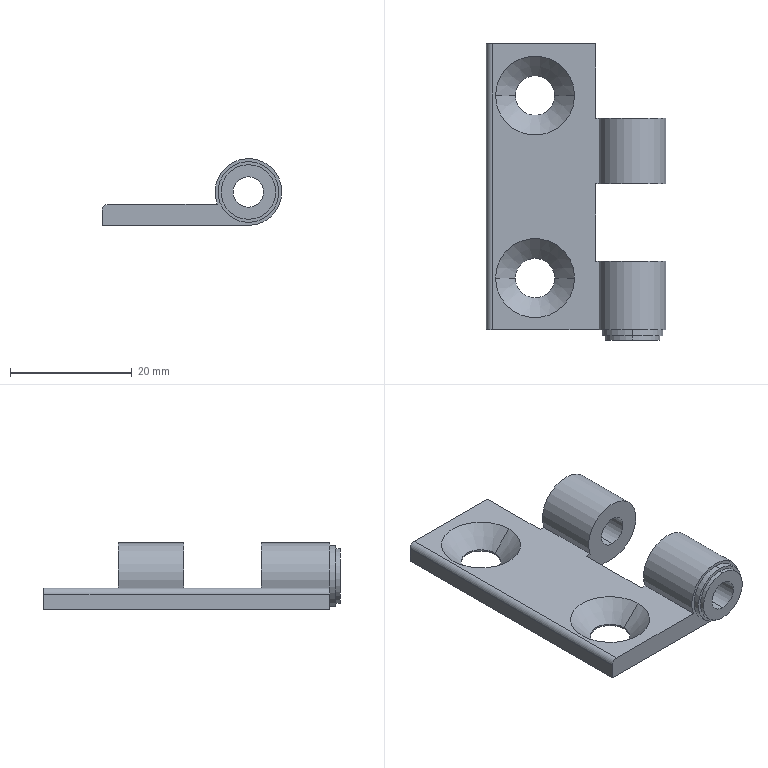Part | STEP file | SecondRearHHPMGS6p1_Default | 1 solid | 31 faces | box 29.5 x 48.7 x 11 mm | volume 4355 mm3 | cylinder 15 | plane 12 | cone 4 | commonest cylinder face diameters 5 x4 6.5 x4 9 x2 10 x2 11 x2 2 x1